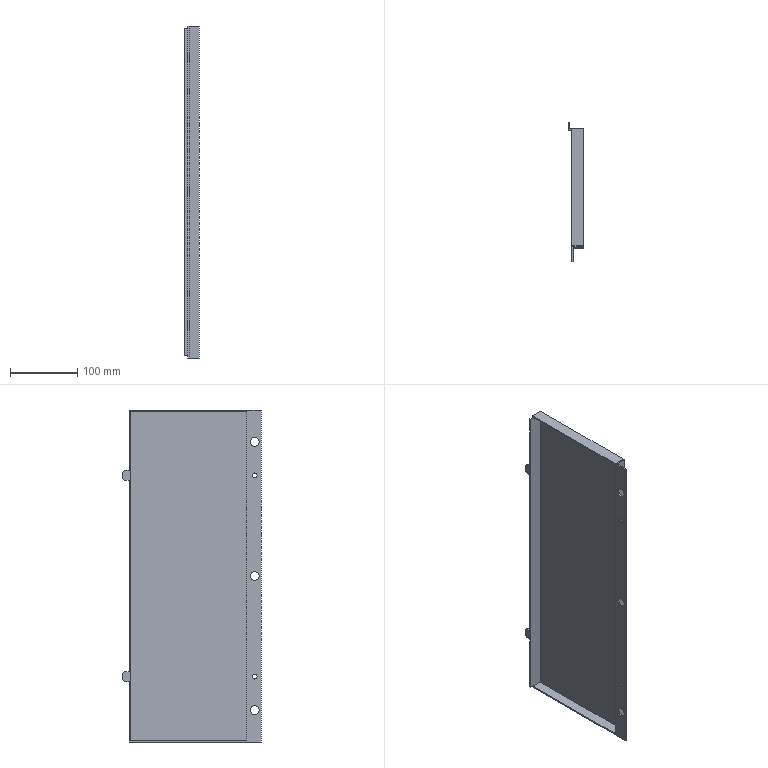Part | SolidWorks | features BaseBody 1 | 1 solid | 42 faces | box 22 x 207 x 495 mm | volume 239502 mm3 | plane 32 | cylinder 10 | commonest cylinder face diameters 13.1 x6 7.2 x4
STEP:
#1=CARTESIAN_POINT('',(194.446,-4330.973,706.371));
#2=VERTEX_POINT('',#1);
#3=CARTESIAN_POINT('',(194.446,-4330.973,713.571));
#4=VERTEX_POINT('',#3);
#5=CARTESIAN_POINT('',(194.446,-4330.973,709.971));
#6=DIRECTION('',(-1.,0.,0.));
#7=DIRECTION('',(0.,0.,1.));
#8=AXIS2_PLACEMENT_3D('',#5,#6,#7);
#9=CIRCLE('',#8,3.6);
#10=EDGE_CURVE('',#2,#4,#9,.T.);
#11=ORIENTED_EDGE('',*,*,#10,.F.);
#12=CARTESIAN_POINT('',(192.446,-4330.973,706.371));
#13=VERTEX_POINT('',#12);
#14=CARTESIAN_POINT('',(201.592,-4330.973,706.371));
#15=DIRECTION('',(-1.,0.,0.));
#16=VECTOR('',#15,1000.);
#17=LINE('',#14,#16);
#18=EDGE_CURVE('',#2,#13,#17,.T.);
#19=ORIENTED_EDGE('',*,*,#18,.T.);
#20=CARTESIAN_POINT('',(192.446,-4330.973,713.571));
#21=VERTEX_POINT('',#20);
#22=CARTESIAN_POINT('',(192.446,-4330.973,709.971));
#23=DIRECTION('',(1.,0.,0.));
#24=DIRECTION('',(0.,0.,1.));
#25=AXIS2_PLACEMENT_3D('',#22,#23,#24);
#26=CIRCLE('',#25,3.6);
#27=EDGE_CURVE('',#21,#13,#26,.T.);
#28=ORIENTED_EDGE('',*,*,#27,.F.);
#29=CARTESIAN_POINT('',(201.592,-4330.973,713.571));
#30=DIRECTION('',(-1.,0.,0.));
#31=VECTOR('',#30,1000.);
#32=LINE('',#29,#31);
#33=EDGE_CURVE('',#4,#21,#32,.T.);
#34=ORIENTED_EDGE('',*,*,#33,.F.);
#35=EDGE_LOOP('',(#11,#19,#28,#34));
#36=FACE_OUTER_BOUND('',#35,.T.);
#37=CARTESIAN_POINT('',(201.592,-4330.973,709.971));
#38=DIRECTION('',(-1.,0.,0.));
#39=DIRECTION('',(0.,0.,1.));
#40=AXIS2_PLACEMENT_3D('',#37,#38,#39);
#41=CYLINDRICAL_SURFACE('',#40,3.6);
#42=ADVANCED_FACE('',(#36),#41,.F.);
#43=CARTESIAN_POINT('',(194.446,-4330.973,406.371));
#44=VERTEX_POINT('',#43);
#45=CARTESIAN_POINT('',(194.446,-4330.973,413.571));
#46=VERTEX_POINT('',#45);
#47=CARTESIAN_POINT('',(194.446,-4330.973,409.971));
#48=DIRECTION('',(-1.,0.,0.));
#49=DIRECTION('',(0.,0.,1.));
#50=AXIS2_PLACEMENT_3D('',#47,#48,#49);
#51=CIRCLE('',#50,3.6);
#52=EDGE_CURVE('',#44,#46,#51,.T.);
#53=ORIENTED_EDGE('',*,*,#52,.F.);
#54=CARTESIAN_POINT('',(192.446,-4330.973,406.371));
#55=VERTEX_POINT('',#54);
#56=CARTESIAN_POINT('',(201.592,-4330.973,406.371));
#57=DIRECTION('',(-1.,0.,0.));
#58=VECTOR('',#57,1000.);
#59=LINE('',#56,#58);
#60=EDGE_CURVE('',#44,#55,#59,.T.);
#61=ORIENTED_EDGE('',*,*,#60,.T.);
#62=CARTESIAN_POINT('',(192.446,-4330.973,413.571));
#63=VERTEX_POINT('',#62);
#64=CARTESIAN_POINT('',(192.446,-4330.973,409.971));
#65=DIRECTION('',(1.,0.,0.));
#66=DIRECTION('',(0.,0.,1.));
#67=AXIS2_PLACEMENT_3D('',#64,#65,#66);
#68=CIRCLE('',#67,3.6);
#69=EDGE_CURVE('',#63,#55,#68,.T.);
#70=ORIENTED_EDGE('',*,*,#69,.F.);
#71=CARTESIAN_POINT('',(201.592,-4330.973,413.571));
#72=DIRECTION('',(-1.,0.,0.));
#73=VECTOR('',#72,1000.);
#74=LINE('',#71,#73);
#75=EDGE_CURVE('',#46,#63,#74,.T.);
#76=ORIENTED_EDGE('',*,*,#75,.F.);
#77=EDGE_LOOP('',(#53,#61,#70,#76));
#78=FACE_OUTER_BOUND('',#77,.T.);
#79=CARTESIAN_POINT('',(201.592,-4330.973,409.971));
#80=DIRECTION('',(-1.,0.,0.));
#81=DIRECTION('',(0.,0.,1.));
#82=AXIS2_PLACEMENT_3D('',#79,#80,#81);
#83=CYLINDRICAL_SURFACE('',#82,3.6);
#84=ADVANCED_FACE('',(#78),#83,.F.);
#85=CARTESIAN_POINT('',(194.446,-4330.973,353.421));
#86=VERTEX_POINT('',#85);
#87=CARTESIAN_POINT('',(194.446,-4330.973,366.521));
#88=VERTEX_POINT('',#87);
#89=CARTESIAN_POINT('',(194.446,-4330.973,359.971));
#90=DIRECTION('',(-1.,0.,0.));
#91=DIRECTION('',(0.,0.,1.));
#92=AXIS2_PLACEMENT_3D('',#89,#90,#91);
#93=CIRCLE('',#92,6.55);
#94=EDGE_CURVE('',#86,#88,#93,.T.);
#95=ORIENTED_EDGE('',*,*,#94,.F.);
#96=CARTESIAN_POINT('',(192.446,-4330.973,353.421));
#97=VERTEX_POINT('',#96);
#98=CARTESIAN_POINT('',(212.499,-4330.973,353.421));
#99=DIRECTION('',(-1.,0.,0.));
#100=VECTOR('',#99,1000.);
#101=LINE('',#98,#100);
#102=EDGE_CURVE('',#86,#97,#101,.T.);
#103=ORIENTED_EDGE('',*,*,#102,.T.);
#104=CARTESIAN_POINT('',(192.446,-4330.973,366.521));
#105=VERTEX_POINT('',#104);
#106=CARTESIAN_POINT('',(192.446,-4330.973,359.971));
#107=DIRECTION('',(1.,0.,0.));
#108=DIRECTION('',(0.,0.,1.));
#109=AXIS2_PLACEMENT_3D('',#106,#107,#108);
#110=CIRCLE('',#109,6.55);
#111=EDGE_CURVE('',#105,#97,#110,.T.);
#112=ORIENTED_EDGE('',*,*,#111,.F.);
#113=CARTESIAN_POINT('',(212.499,-4330.973,366.521));
#114=DIRECTION('',(-1.,0.,0.));
#115=VECTOR('',#114,1000.);
#116=LINE('',#113,#115);
#117=EDGE_CURVE('',#88,#105,#116,.T.);
#118=ORIENTED_EDGE('',*,*,#117,.F.);
#119=EDGE_LOOP('',(#95,#103,#112,#118));
#120=FACE_OUTER_BOUND('',#119,.T.);
#121=CARTESIAN_POINT('',(212.499,-4330.973,359.971));
#122=DIRECTION('',(-1.,0.,0.));
#123=DIRECTION('',(0.,0.,1.));
#124=AXIS2_PLACEMENT_3D('',#121,#122,#123);
#125=CYLINDRICAL_SURFACE('',#124,6.55);
#126=ADVANCED_FACE('',(#120),#125,.F.);
#127=CARTESIAN_POINT('',(194.446,-4330.973,753.421));
#128=VERTEX_POINT('',#127);
#129=CARTESIAN_POINT('',(194.446,-4330.973,766.521));
#130=VERTEX_POINT('',#129);
#131=CARTESIAN_POINT('',(194.446,-4330.973,759.971));
#132=DIRECTION('',(-1.,0.,0.));
#133=DIRECTION('',(0.,0.,1.));
#134=AXIS2_PLACEMENT_3D('',#131,#132,#133);
#135=CIRCLE('',#134,6.55);
#136=EDGE_CURVE('',#128,#130,#135,.T.);
#137=ORIENTED_EDGE('',*,*,#136,.F.);
#138=CARTESIAN_POINT('',(192.446,-4330.973,753.421));
#139=VERTEX_POINT('',#138);
#140=CARTESIAN_POINT('',(210.499,-4330.973,753.421));
#141=DIRECTION('',(-1.,0.,0.));
#142=VECTOR('',#141,1000.);
#143=LINE('',#140,#142);
#144=EDGE_CURVE('',#128,#139,#143,.T.);
#145=ORIENTED_EDGE('',*,*,#144,.T.);
#146=CARTESIAN_POINT('',(192.446,-4330.973,766.521));
#147=VERTEX_POINT('',#146);
#148=CARTESIAN_POINT('',(192.446,-4330.973,759.971));
#149=DIRECTION('',(1.,0.,0.));
#150=DIRECTION('',(0.,0.,1.));
#151=AXIS2_PLACEMENT_3D('',#148,#149,#150);
#152=CIRCLE('',#151,6.55);
#153=EDGE_CURVE('',#147,#139,#152,.T.);
#154=ORIENTED_EDGE('',*,*,#153,.F.);
#155=CARTESIAN_POINT('',(210.499,-4330.973,766.521));
#156=DIRECTION('',(-1.,0.,0.));
#157=VECTOR('',#156,1000.);
#158=LINE('',#155,#157);
#159=EDGE_CURVE('',#130,#147,#158,.T.);
#160=ORIENTED_EDGE('',*,*,#159,.F.);
#161=EDGE_LOOP('',(#137,#145,#154,#160));
#162=FACE_OUTER_BOUND('',#161,.T.);
#163=CARTESIAN_POINT('',(210.499,-4330.973,759.971));
#164=DIRECTION('',(-1.,0.,0.));
#165=DIRECTION('',(0.,0.,1.));
#166=AXIS2_PLACEMENT_3D('',#163,#164,#165);
#167=CYLINDRICAL_SURFACE('',#166,6.55);
#168=ADVANCED_FACE('',(#162),#167,.F.);
#169=CARTESIAN_POINT('',(194.446,-4330.973,553.421));
#170=VERTEX_POINT('',#169);
#171=CARTESIAN_POINT('',(194.446,-4330.973,566.521));
#172=VERTEX_POINT('',#171);
#173=CARTESIAN_POINT('',(194.446,-4330.973,559.971));
#174=DIRECTION('',(-1.,0.,0.));
#175=DIRECTION('',(0.,0.,1.));
#176=AXIS2_PLACEMENT_3D('',#173,#174,#175);
#177=CIRCLE('',#176,6.55);
#178=EDGE_CURVE('',#170,#172,#177,.T.);
#179=ORIENTED_EDGE('',*,*,#178,.F.);
#180=CARTESIAN_POINT('',(192.446,-4330.973,553.421));
#181=VERTEX_POINT('',#180);
#182=CARTESIAN_POINT('',(212.499,-4330.973,553.421));
#183=DIRECTION('',(-1.,0.,0.));
#184=VECTOR('',#183,1000.);
#185=LINE('',#182,#184);
#186=EDGE_CURVE('',#170,#181,#185,.T.);
#187=ORIENTED_EDGE('',*,*,#186,.T.);
#188=CARTESIAN_POINT('',(192.446,-4330.973,566.521));
#189=VERTEX_POINT('',#188);
#190=CARTESIAN_POINT('',(192.446,-4330.973,559.971));
#191=DIRECTION('',(1.,0.,0.));
#192=DIRECTION('',(0.,0.,1.));
#193=AXIS2_PLACEMENT_3D('',#190,#191,#192);
#194=CIRCLE('',#193,6.55);
#195=EDGE_CURVE('',#189,#181,#194,.T.);
#196=ORIENTED_EDGE('',*,*,#195,.F.);
#197=CARTESIAN_POINT('',(212.499,-4330.973,566.521));
#198=DIRECTION('',(-1.,0.,0.));
#199=VECTOR('',#198,1000.);
#200=LINE('',#197,#199);
#201=EDGE_CURVE('',#172,#189,#200,.T.);
#202=ORIENTED_EDGE('',*,*,#201,.F.);
#203=EDGE_LOOP('',(#179,#187,#196,#202));
#204=FACE_OUTER_BOUND('',#203,.T.);
#205=CARTESIAN_POINT('',(212.499,-4330.973,559.971));
#206=DIRECTION('',(-1.,0.,0.));
#207=DIRECTION('',(0.,0.,1.));
#208=AXIS2_PLACEMENT_3D('',#205,#206,#207);
#209=CYLINDRICAL_SURFACE('',#208,6.55);
#210=ADVANCED_FACE('',(#204),#209,.F.);
#211=CARTESIAN_POINT('',(209.446,-4320.973,312.471));
#212=VERTEX_POINT('',#211);
#213=CARTESIAN_POINT('',(209.446,-4143.973,312.471));
#214=VERTEX_POINT('',#213);
#215=CARTESIAN_POINT('',(209.446,-4143.973,312.471));
#216=DIRECTION('',(0.,1.,0.));
#217=VECTOR('',#216,1000.);
#218=LINE('',#215,#217);
#219=EDGE_CURVE('',#212,#214,#218,.T.);
#220=ORIENTED_EDGE('',*,*,#219,.T.);
#221=CARTESIAN_POINT('',(209.446,-4143.973,807.471));
#222=VERTEX_POINT('',#221);
#223=CARTESIAN_POINT('',(209.446,-4143.973,207.471));
#224=DIRECTION('',(0.,0.,1.));
#225=VECTOR('',#224,1000.);
#226=LINE('',#223,#225);
#227=EDGE_CURVE('',#214,#222,#226,.T.);
#228=ORIENTED_EDGE('',*,*,#227,.T.);
#229=CARTESIAN_POINT('',(209.446,-4320.973,807.471));
#230=VERTEX_POINT('',#229);
#231=CARTESIAN_POINT('',(209.446,-4143.973,807.471));
#232=DIRECTION('',(0.,-1.,0.));
#233=VECTOR('',#232,1000.);
#234=LINE('',#231,#233);
#235=EDGE_CURVE('',#222,#230,#234,.T.);
#236=ORIENTED_EDGE('',*,*,#235,.T.);
#237=CARTESIAN_POINT('',(209.446,-4320.973,207.471));
#238=DIRECTION('',(0.,0.,-1.));
#239=VECTOR('',#238,1000.);
#240=LINE('',#237,#239);
#241=EDGE_CURVE('',#230,#212,#240,.T.);
#242=ORIENTED_EDGE('',*,*,#241,.T.);
#243=EDGE_LOOP('',(#220,#228,#236,#242));
#244=FACE_OUTER_BOUND('',#243,.T.);
#245=CARTESIAN_POINT('',(209.446,-4143.973,207.471));
#246=DIRECTION('',(1.,0.,0.));
#247=DIRECTION('',(0.,0.,-1.));
#248=AXIS2_PLACEMENT_3D('',#245,#246,#247);
#249=PLANE('',#248);
#250=ADVANCED_FACE('',(#244),#249,.T.);
#251=CARTESIAN_POINT('',(187.446,-4143.973,402.471));
#252=VERTEX_POINT('',#251);
#253=CARTESIAN_POINT('',(189.446,-4143.973,402.471));
#254=VERTEX_POINT('',#253);
#255=CARTESIAN_POINT('',(207.446,-4143.973,402.471));
#256=DIRECTION('',(1.,0.,0.));
#257=VECTOR('',#256,1000.);
#258=LINE('',#255,#257);
#259=EDGE_CURVE('',#252,#254,#258,.T.);
#260=ORIENTED_EDGE('',*,*,#259,.T.);
#261=CARTESIAN_POINT('',(189.446,-4143.973,417.471));
#262=VERTEX_POINT('',#261);
#263=CARTESIAN_POINT('',(189.446,-4143.973,910.471));
#264=DIRECTION('',(0.,0.,1.));
#265=VECTOR('',#264,1000.);
#266=LINE('',#263,#265);
#267=EDGE_CURVE('',#254,#262,#266,.T.);
#268=ORIENTED_EDGE('',*,*,#267,.T.);
#269=CARTESIAN_POINT('',(187.446,-4143.973,417.471));
#270=VERTEX_POINT('',#269);
#271=CARTESIAN_POINT('',(207.446,-4143.973,417.471));
#272=DIRECTION('',(-1.,0.,0.));
#273=VECTOR('',#272,1000.);
#274=LINE('',#271,#273);
#275=EDGE_CURVE('',#262,#270,#274,.T.);
#276=ORIENTED_EDGE('',*,*,#275,.T.);
#277=CARTESIAN_POINT('',(187.446,-4143.973,702.471));
#278=VERTEX_POINT('',#277);
#279=CARTESIAN_POINT('',(187.446,-4143.973,910.471));
#280=DIRECTION('',(0.,0.,1.));
#281=VECTOR('',#280,1000.);
#282=LINE('',#279,#281);
#283=EDGE_CURVE('',#270,#278,#282,.T.);
#284=ORIENTED_EDGE('',*,*,#283,.T.);
#285=CARTESIAN_POINT('',(189.446,-4143.973,702.471));
#286=VERTEX_POINT('',#285);
#287=CARTESIAN_POINT('',(207.446,-4143.973,702.471));
#288=DIRECTION('',(1.,0.,0.));
#289=VECTOR('',#288,1000.);
#290=LINE('',#287,#289);
#291=EDGE_CURVE('',#278,#286,#290,.T.);
#292=ORIENTED_EDGE('',*,*,#291,.T.);
#293=CARTESIAN_POINT('',(189.446,-4143.973,717.471));
#294=VERTEX_POINT('',#293);
#295=CARTESIAN_POINT('',(189.446,-4143.973,910.471));
#296=DIRECTION('',(0.,0.,1.));
#297=VECTOR('',#296,1000.);
#298=LINE('',#295,#297);
#299=EDGE_CURVE('',#286,#294,#298,.T.);
#300=ORIENTED_EDGE('',*,*,#299,.T.);
#301=CARTESIAN_POINT('',(187.446,-4143.973,717.471));
#302=VERTEX_POINT('',#301);
#303=CARTESIAN_POINT('',(207.446,-4143.973,717.471));
#304=DIRECTION('',(-1.,0.,0.));
#305=VECTOR('',#304,1000.);
#306=LINE('',#303,#305);
#307=EDGE_CURVE('',#294,#302,#306,.T.);
#308=ORIENTED_EDGE('',*,*,#307,.T.);
#309=CARTESIAN_POINT('',(187.446,-4143.973,804.471));
#310=VERTEX_POINT('',#309);
#311=CARTESIAN_POINT('',(187.446,-4143.973,910.471));
#312=DIRECTION('',(0.,0.,1.));
#313=VECTOR('',#312,1000.);
#314=LINE('',#311,#313);
#315=EDGE_CURVE('',#302,#310,#314,.T.);
#316=ORIENTED_EDGE('',*,*,#315,.T.);
#317=CARTESIAN_POINT('',(207.446,-4143.973,804.471));
#318=VERTEX_POINT('',#317);
#319=CARTESIAN_POINT('',(207.446,-4143.973,804.471));
#320=DIRECTION('',(1.,0.,0.));
#321=VECTOR('',#320,1000.);
#322=LINE('',#319,#321);
#323=EDGE_CURVE('',#310,#318,#322,.T.);
#324=ORIENTED_EDGE('',*,*,#323,.T.);
#325=CARTESIAN_POINT('',(207.446,-4143.973,805.471));
#326=VERTEX_POINT('',#325);
#327=CARTESIAN_POINT('',(207.446,-4143.973,207.471));
#328=DIRECTION('',(0.,0.,-1.));
#329=VECTOR('',#328,1000.);
#330=LINE('',#327,#329);
#331=EDGE_CURVE('',#326,#318,#330,.T.);
#332=ORIENTED_EDGE('',*,*,#331,.F.);
#333=CARTESIAN_POINT('',(192.446,-4143.973,805.471));
#334=VERTEX_POINT('',#333);
#335=CARTESIAN_POINT('',(207.446,-4143.973,805.471));
#336=DIRECTION('',(-1.,0.,0.));
#337=VECTOR('',#336,1000.);
#338=LINE('',#335,#337);
#339=EDGE_CURVE('',#326,#334,#338,.T.);
#340=ORIENTED_EDGE('',*,*,#339,.T.);
#341=CARTESIAN_POINT('',(192.446,-4143.973,807.471));
#342=VERTEX_POINT('',#341);
#343=CARTESIAN_POINT('',(192.446,-4143.973,910.471));
#344=DIRECTION('',(0.,0.,1.));
#345=VECTOR('',#344,1000.);
#346=LINE('',#343,#345);
#347=EDGE_CURVE('',#334,#342,#346,.T.);
#348=ORIENTED_EDGE('',*,*,#347,.T.);
#349=CARTESIAN_POINT('',(207.446,-4143.973,807.471));
#350=DIRECTION('',(1.,0.,0.));
#351=VECTOR('',#350,1000.);
#352=LINE('',#349,#351);
#353=EDGE_CURVE('',#342,#222,#352,.T.);
#354=ORIENTED_EDGE('',*,*,#353,.T.);
#355=ORIENTED_EDGE('',*,*,#227,.F.);
#356=CARTESIAN_POINT('',(192.446,-4143.973,312.471));
#357=VERTEX_POINT('',#356);
#358=CARTESIAN_POINT('',(207.446,-4143.973,312.471));
#359=DIRECTION('',(-1.,0.,0.));
#360=VECTOR('',#359,1000.);
#361=LINE('',#358,#360);
#362=EDGE_CURVE('',#214,#357,#361,.T.);
#363=ORIENTED_EDGE('',*,*,#362,.T.);
#364=CARTESIAN_POINT('',(192.446,-4143.973,314.471));
#365=VERTEX_POINT('',#364);
#366=CARTESIAN_POINT('',(192.446,-4143.973,910.471));
#367=DIRECTION('',(0.,0.,1.));
#368=VECTOR('',#367,1000.);
#369=LINE('',#366,#368);
#370=EDGE_CURVE('',#357,#365,#369,.T.);
#371=ORIENTED_EDGE('',*,*,#370,.T.);
#372=CARTESIAN_POINT('',(207.446,-4143.973,314.471));
#373=VERTEX_POINT('',#372);
#374=CARTESIAN_POINT('',(207.446,-4143.973,314.471));
#375=DIRECTION('',(1.,0.,0.));
#376=VECTOR('',#375,1000.);
#377=LINE('',#374,#376);
#378=EDGE_CURVE('',#365,#373,#377,.T.);
#379=ORIENTED_EDGE('',*,*,#378,.T.);
#380=CARTESIAN_POINT('',(207.446,-4143.973,315.471));
#381=VERTEX_POINT('',#380);
#382=CARTESIAN_POINT('',(207.446,-4143.973,207.471));
#383=DIRECTION('',(0.,0.,-1.));
#384=VECTOR('',#383,1000.);
#385=LINE('',#382,#384);
#386=EDGE_CURVE('',#381,#373,#385,.T.);
#387=ORIENTED_EDGE('',*,*,#386,.F.);
#388=CARTESIAN_POINT('',(187.446,-4143.973,315.471));
#389=VERTEX_POINT('',#388);
#390=CARTESIAN_POINT('',(207.446,-4143.973,315.471));
#391=DIRECTION('',(-1.,0.,0.));
#392=VECTOR('',#391,1000.);
#393=LINE('',#390,#392);
#394=EDGE_CURVE('',#381,#389,#393,.T.);
#395=ORIENTED_EDGE('',*,*,#394,.T.);
#396=CARTESIAN_POINT('',(187.446,-4143.973,910.471));
#397=DIRECTION('',(0.,0.,1.));
#398=VECTOR('',#397,1000.);
#399=LINE('',#396,#398);
#400=EDGE_CURVE('',#389,#252,#399,.T.);
#401=ORIENTED_EDGE('',*,*,#400,.T.);
#402=EDGE_LOOP('',(#260,#268,#276,#284,#292,#300,#308,#316,#324,#332,#340,#348,#354,#355,#363,#371,#379,#387,#395,#401));
#403=FACE_OUTER_BOUND('',#402,.T.);
#404=CARTESIAN_POINT('',(207.446,-4143.973,910.471));
#405=DIRECTION('',(0.,1.,0.));
#406=DIRECTION('',(0.,0.,1.));
#407=AXIS2_PLACEMENT_3D('',#404,#405,#406);
#408=PLANE('',#407);
#409=ADVANCED_FACE('',(#403),#408,.T.);
#410=CARTESIAN_POINT('',(207.446,-4318.473,312.471));
#411=VERTEX_POINT('',#410);
#412=CARTESIAN_POINT('',(207.446,-4318.973,312.471));
#413=VERTEX_POINT('',#412);
#414=CARTESIAN_POINT('',(207.446,-4318.973,312.471));
#415=DIRECTION('',(0.,-1.,0.));
#416=VECTOR('',#415,1000.);
#417=LINE('',#414,#416);
#418=EDGE_CURVE('',#411,#413,#417,.T.);
#419=ORIENTED_EDGE('',*,*,#418,.F.);
#420=CARTESIAN_POINT('',(192.446,-4318.473,312.471));
#421=VERTEX_POINT('',#420);
#422=CARTESIAN_POINT('',(207.446,-4318.473,312.471));
#423=DIRECTION('',(-1.,0.,0.));
#424=VECTOR('',#423,1000.);
#425=LINE('',#422,#424);
#426=EDGE_CURVE('',#411,#421,#425,.T.);
#427=ORIENTED_EDGE('',*,*,#426,.T.);
#428=CARTESIAN_POINT('',(192.446,-4143.973,312.471));
#429=DIRECTION('',(0.,1.,0.));
#430=VECTOR('',#429,1000.);
#431=LINE('',#428,#430);
#432=EDGE_CURVE('',#421,#357,#431,.T.);
#433=ORIENTED_EDGE('',*,*,#432,.T.);
#434=ORIENTED_EDGE('',*,*,#362,.F.);
#435=ORIENTED_EDGE('',*,*,#219,.F.);
#436=CARTESIAN_POINT('',(194.446,-4320.973,312.471));
#437=VERTEX_POINT('',#436);
#438=CARTESIAN_POINT('',(207.446,-4320.973,312.471));
#439=DIRECTION('',(-1.,0.,0.));
#440=VECTOR('',#439,1000.);
#441=LINE('',#438,#440);
#442=EDGE_CURVE('',#212,#437,#441,.T.);
#443=ORIENTED_EDGE('',*,*,#442,.T.);
#444=CARTESIAN_POINT('',(194.446,-4340.973,312.471));
#445=VERTEX_POINT('',#444);
#446=CARTESIAN_POINT('',(194.446,-4143.973,312.471));
#447=DIRECTION('',(0.,-1.,0.));
#448=VECTOR('',#447,1000.);
#449=LINE('',#446,#448);
#450=EDGE_CURVE('',#437,#445,#449,.T.);
#451=ORIENTED_EDGE('',*,*,#450,.T.);
#452=CARTESIAN_POINT('',(192.446,-4340.973,312.471));
#453=VERTEX_POINT('',#452);
#454=CARTESIAN_POINT('',(207.446,-4340.973,312.471));
#455=DIRECTION('',(-1.,0.,0.));
#456=VECTOR('',#455,1000.);
#457=LINE('',#454,#456);
#458=EDGE_CURVE('',#445,#453,#457,.T.);
#459=ORIENTED_EDGE('',*,*,#458,.T.);
#460=CARTESIAN_POINT('',(192.446,-4318.973,312.471));
#461=VERTEX_POINT('',#460);
#462=CARTESIAN_POINT('',(192.446,-4143.973,312.471));
#463=DIRECTION('',(0.,1.,0.));
#464=VECTOR('',#463,1000.);
#465=LINE('',#462,#464);
#466=EDGE_CURVE('',#453,#461,#465,.T.);
#467=ORIENTED_EDGE('',*,*,#466,.T.);
#468=CARTESIAN_POINT('',(207.446,-4318.973,312.471));
#469=DIRECTION('',(1.,0.,0.));
#470=VECTOR('',#469,1000.);
#471=LINE('',#468,#470);
#472=EDGE_CURVE('',#461,#413,#471,.T.);
#473=ORIENTED_EDGE('',*,*,#472,.T.);
#474=EDGE_LOOP('',(#419,#427,#433,#434,#435,#443,#451,#459,#467,#473));
#475=FACE_OUTER_BOUND('',#474,.T.);
#476=CARTESIAN_POINT('',(207.446,-4143.973,312.471));
#477=DIRECTION('',(0.,0.,-1.));
#478=DIRECTION('',(-1.,0.,0.));
#479=AXIS2_PLACEMENT_3D('',#476,#477,#478);
#480=PLANE('',#479);
#481=ADVANCED_FACE('',(#475),#480,.T.);
#482=ORIENTED_EDGE('',*,*,#442,.F.);
#483=ORIENTED_EDGE('',*,*,#241,.F.);
#484=CARTESIAN_POINT('',(194.446,-4320.973,807.471));
#485=VERTEX_POINT('',#484);
#486=CARTESIAN_POINT('',(209.446,-4320.973,807.471));
#487=DIRECTION('',(-1.,0.,0.));
#488=VECTOR('',#487,1000.);
#489=LINE('',#486,#488);
#490=EDGE_CURVE('',#230,#485,#489,.T.);
#491=ORIENTED_EDGE('',*,*,#490,.T.);
#492=CARTESIAN_POINT('',(194.446,-4320.973,207.471));
#493=DIRECTION('',(0.,0.,-1.));
#494=VECTOR('',#493,1000.);
#495=LINE('',#492,#494);
#496=EDGE_CURVE('',#485,#437,#495,.T.);
#497=ORIENTED_EDGE('',*,*,#496,.T.);
#498=EDGE_LOOP('',(#482,#483,#491,#497));
#499=FACE_OUTER_BOUND('',#498,.T.);
#500=CARTESIAN_POINT('',(209.446,-4320.973,207.471));
#501=DIRECTION('',(0.,-1.,0.));
#502=DIRECTION('',(0.,0.,-1.));
#503=AXIS2_PLACEMENT_3D('',#500,#501,#502);
#504=PLANE('',#503);
#505=ADVANCED_FACE('',(#499),#504,.T.);
#506=ORIENTED_EDGE('',*,*,#235,.F.);
#507=ORIENTED_EDGE('',*,*,#353,.F.);
#508=CARTESIAN_POINT('',(192.446,-4318.473,807.471));
#509=VERTEX_POINT('',#508);
#510=CARTESIAN_POINT('',(192.446,-4143.973,807.471));
#511=DIRECTION('',(0.,-1.,0.));
#512=VECTOR('',#511,1000.);
#513=LINE('',#510,#512);
#514=EDGE_CURVE('',#342,#509,#513,.T.);
#515=ORIENTED_EDGE('',*,*,#514,.T.);
#516=CARTESIAN_POINT('',(207.446,-4318.473,807.471));
#517=VERTEX_POINT('',#516);
#518=CARTESIAN_POINT('',(207.446,-4318.473,807.471));
#519=DIRECTION('',(1.,0.,0.));
#520=VECTOR('',#519,1000.);
#521=LINE('',#518,#520);
#522=EDGE_CURVE('',#509,#517,#521,.T.);
#523=ORIENTED_EDGE('',*,*,#522,.T.);
#524=CARTESIAN_POINT('',(207.446,-4318.973,807.471));
#525=VERTEX_POINT('',#524);
#526=CARTESIAN_POINT('',(207.446,-4318.973,807.471));
#527=DIRECTION('',(0.,1.,0.));
#528=VECTOR('',#527,1000.);
#529=LINE('',#526,#528);
#530=EDGE_CURVE('',#525,#517,#529,.T.);
#531=ORIENTED_EDGE('',*,*,#530,.F.);
#532=CARTESIAN_POINT('',(192.446,-4318.973,807.471));
#533=VERTEX_POINT('',#532);
#534=CARTESIAN_POINT('',(207.446,-4318.973,807.471));
#535=DIRECTION('',(-1.,0.,0.));
#536=VECTOR('',#535,1000.);
#537=LINE('',#534,#536);
#538=EDGE_CURVE('',#525,#533,#537,.T.);
#539=ORIENTED_EDGE('',*,*,#538,.T.);
#540=CARTESIAN_POINT('',(192.446,-4340.973,807.471));
#541=VERTEX_POINT('',#540);
#542=CARTESIAN_POINT('',(192.446,-4143.973,807.471));
#543=DIRECTION('',(0.,-1.,0.));
#544=VECTOR('',#543,1000.);
#545=LINE('',#542,#544);
#546=EDGE_CURVE('',#533,#541,#545,.T.);
#547=ORIENTED_EDGE('',*,*,#546,.T.);
#548=CARTESIAN_POINT('',(194.446,-4340.973,807.471));
#549=VERTEX_POINT('',#548);
#550=CARTESIAN_POINT('',(207.446,-4340.973,807.471));
#551=DIRECTION('',(1.,0.,0.));
#552=VECTOR('',#551,1000.);
#553=LINE('',#550,#552);
#554=EDGE_CURVE('',#541,#549,#553,.T.);
#555=ORIENTED_EDGE('',*,*,#554,.T.);
#556=CARTESIAN_POINT('',(194.446,-4143.973,807.471));
#557=DIRECTION('',(0.,1.,0.));
#558=VECTOR('',#557,1000.);
#559=LINE('',#556,#558);
#560=EDGE_CURVE('',#549,#485,#559,.T.);
#561=ORIENTED_EDGE('',*,*,#560,.T.);
#562=ORIENTED_EDGE('',*,*,#490,.F.);
#563=EDGE_LOOP('',(#506,#507,#515,#523,#531,#539,#547,#555,#561,#562));
#564=FACE_OUTER_BOUND('',#563,.T.);
#565=CARTESIAN_POINT('',(207.446,-4143.973,807.471));
#566=DIRECTION('',(0.,0.,1.));
#567=DIRECTION('',(1.,0.,0.));
#568=AXIS2_PLACEMENT_3D('',#565,#566,#567);
#569=PLANE('',#568);
#570=ADVANCED_FACE('',(#564),#569,.T.);
#571=CARTESIAN_POINT('',(189.446,-4133.973,414.471));
#572=VERTEX_POINT('',#571);
#573=CARTESIAN_POINT('',(189.446,-4136.973,417.471));
#574=VERTEX_POINT('',#573);
#575=CARTESIAN_POINT('',(189.446,-4133.973,414.471));
#576=DIRECTION('',(0.,-0.7071,0.7071));
#577=VECTOR('',#576,1000.);
#578=LINE('',#575,#577);
#579=EDGE_CURVE('',#572,#574,#578,.T.);
#580=ORIENTED_EDGE('',*,*,#579,.T.);
#581=CARTESIAN_POINT('',(189.446,-4140.465,417.471));
#582=DIRECTION('',(0.,-1.,0.));
#583=VECTOR('',#582,1000.);
#584=LINE('',#581,#583);
#585=EDGE_CURVE('',#574,#262,#584,.T.);
#586=ORIENTED_EDGE('',*,*,#585,.T.);
#587=ORIENTED_EDGE('',*,*,#267,.F.);
#588=CARTESIAN_POINT('',(189.446,-4136.973,402.471));
#589=VERTEX_POINT('',#588);
#590=CARTESIAN_POINT('',(189.446,-4140.465,402.471));
#591=DIRECTION('',(0.,1.,0.));
#592=VECTOR('',#591,1000.);
#593=LINE('',#590,#592);
#594=EDGE_CURVE('',#254,#589,#593,.T.);
#595=ORIENTED_EDGE('',*,*,#594,.T.);
#596=CARTESIAN_POINT('',(189.446,-4133.973,405.471));
#597=VERTEX_POINT('',#596);
#598=CARTESIAN_POINT('',(189.446,-4136.973,402.471));
#599=DIRECTION('',(0.,0.7071,0.7071));
#600=VECTOR('',#599,1000.);
#601=LINE('',#598,#600);
#602=EDGE_CURVE('',#589,#597,#601,.T.);
#603=ORIENTED_EDGE('',*,*,#602,.T.);
#604=CARTESIAN_POINT('',(189.446,-4133.973,439.971));
#605=DIRECTION('',(0.,0.,1.));
#606=VECTOR('',#605,1000.);
#607=LINE('',#604,#606);
#608=EDGE_CURVE('',#597,#572,#607,.T.);
#609=ORIENTED_EDGE('',*,*,#608,.T.);
#610=EDGE_LOOP('',(#580,#586,#587,#595,#603,#609));
#611=FACE_OUTER_BOUND('',#610,.T.);
#612=CARTESIAN_POINT('',(189.446,-4140.465,439.971));
#613=DIRECTION('',(1.,0.,0.));
#614=DIRECTION('',(0.,0.,-1.));
#615=AXIS2_PLACEMENT_3D('',#612,#613,#614);
#616=PLANE('',#615);
#617=ADVANCED_FACE('',(#611),#616,.T.);
#618=CARTESIAN_POINT('',(187.446,-4136.973,402.471));
#619=VERTEX_POINT('',#618);
#620=CARTESIAN_POINT('',(189.446,-4136.973,402.471));
#621=DIRECTION('',(1.,0.,0.));
#622=VECTOR('',#621,1000.);
#623=LINE('',#620,#622);
#624=EDGE_CURVE('',#619,#589,#623,.T.);
#625=ORIENTED_EDGE('',*,*,#624,.T.);
#626=ORIENTED_EDGE('',*,*,#594,.F.);
#627=ORIENTED_EDGE('',*,*,#259,.F.);
#628=CARTESIAN_POINT('',(187.446,-4145.973,402.471));
#629=DIRECTION('',(0.,1.,0.));
#630=VECTOR('',#629,1000.);
#631=LINE('',#628,#630);
#632=EDGE_CURVE('',#252,#619,#631,.T.);
#633=ORIENTED_EDGE('',*,*,#632,.T.);
#634=EDGE_LOOP('',(#625,#626,#627,#633));
#635=FACE_OUTER_BOUND('',#634,.T.);
#636=CARTESIAN_POINT('',(189.446,-4145.973,402.471));
#637=DIRECTION('',(0.,0.,-1.));
#638=DIRECTION('',(-1.,0.,0.));
#639=AXIS2_PLACEMENT_3D('',#636,#637,#638);
#640=PLANE('',#639);
#641=ADVANCED_FACE('',(#635),#640,.T.);
#642=CARTESIAN_POINT('',(187.446,-4133.973,414.471));
#643=VERTEX_POINT('',#642);
#644=CARTESIAN_POINT('',(187.446,-4136.973,417.471));
#645=VERTEX_POINT('',#644);
#646=CARTESIAN_POINT('',(187.446,-4133.973,414.471));
#647=DIRECTION('',(0.,-0.7071,0.7071));
#648=VECTOR('',#647,1000.);
#649=LINE('',#646,#648);
#650=EDGE_CURVE('',#643,#645,#649,.T.);
#651=ORIENTED_EDGE('',*,*,#650,.F.);
#652=CARTESIAN_POINT('',(187.446,-4133.973,405.471));
#653=VERTEX_POINT('',#652);
#654=CARTESIAN_POINT('',(187.446,-4133.973,484.971));
#655=DIRECTION('',(0.,0.,1.));
#656=VECTOR('',#655,1000.);
#657=LINE('',#654,#656);
#658=EDGE_CURVE('',#653,#643,#657,.T.);
#659=ORIENTED_EDGE('',*,*,#658,.F.);
#660=CARTESIAN_POINT('',(187.446,-4136.973,402.471));
#661=DIRECTION('',(0.,0.7071,0.7071));
#662=VECTOR('',#661,1000.);
#663=LINE('',#660,#662);
#664=EDGE_CURVE('',#619,#653,#663,.T.);
#665=ORIENTED_EDGE('',*,*,#664,.F.);
#666=ORIENTED_EDGE('',*,*,#632,.F.);
#667=ORIENTED_EDGE('',*,*,#400,.F.);
#668=CARTESIAN_POINT('',(187.446,-4145.973,315.471));
#669=VERTEX_POINT('',#668);
#670=CARTESIAN_POINT('',(187.446,-4140.465,315.471));
#671=DIRECTION('',(0.,1.,0.));
#672=VECTOR('',#671,1000.);
#673=LINE('',#670,#672);
#674=EDGE_CURVE('',#669,#389,#673,.T.);
#675=ORIENTED_EDGE('',*,*,#674,.F.);
#676=CARTESIAN_POINT('',(187.446,-4145.973,804.471));
#677=VERTEX_POINT('',#676);
#678=CARTESIAN_POINT('',(187.446,-4145.973,484.971));
#679=DIRECTION('',(0.,0.,-1.));
#680=VECTOR('',#679,1000.);
#681=LINE('',#678,#680);
#682=EDGE_CURVE('',#677,#669,#681,.T.);
#683=ORIENTED_EDGE('',*,*,#682,.F.);
#684=CARTESIAN_POINT('',(187.446,-4140.465,804.471));
#685=DIRECTION('',(0.,-1.,0.));
#686=VECTOR('',#685,1000.);
#687=LINE('',#684,#686);
#688=EDGE_CURVE('',#310,#677,#687,.T.);
#689=ORIENTED_EDGE('',*,*,#688,.F.);
#690=ORIENTED_EDGE('',*,*,#315,.F.);
#691=CARTESIAN_POINT('',(187.446,-4136.973,717.471));
#692=VERTEX_POINT('',#691);
#693=CARTESIAN_POINT('',(187.446,-4140.465,717.471));
#694=DIRECTION('',(0.,-1.,0.));
#695=VECTOR('',#694,1000.);
#696=LINE('',#693,#695);
#697=EDGE_CURVE('',#692,#302,#696,.T.);
#698=ORIENTED_EDGE('',*,*,#697,.F.);
#699=CARTESIAN_POINT('',(187.446,-4133.973,714.471));
#700=VERTEX_POINT('',#699);
#701=CARTESIAN_POINT('',(187.446,-4133.973,714.471));
#702=DIRECTION('',(0.,-0.7071,0.7071));
#703=VECTOR('',#702,1000.);
#704=LINE('',#701,#703);
#705=EDGE_CURVE('',#700,#692,#704,.T.);
#706=ORIENTED_EDGE('',*,*,#705,.F.);
#707=CARTESIAN_POINT('',(187.446,-4133.973,705.471));
#708=VERTEX_POINT('',#707);
#709=CARTESIAN_POINT('',(187.446,-4133.973,484.971));
#710=DIRECTION('',(0.,0.,1.));
#711=VECTOR('',#710,1000.);
#712=LINE('',#709,#711);
#713=EDGE_CURVE('',#708,#700,#712,.T.);
#714=ORIENTED_EDGE('',*,*,#713,.F.);
#715=CARTESIAN_POINT('',(187.446,-4136.973,702.471));
#716=VERTEX_POINT('',#715);
#717=CARTESIAN_POINT('',(187.446,-4136.973,702.471));
#718=DIRECTION('',(0.,0.7071,0.7071));
#719=VECTOR('',#718,1000.);
#720=LINE('',#717,#719);
#721=EDGE_CURVE('',#716,#708,#720,.T.);
#722=ORIENTED_EDGE('',*,*,#721,.F.);
#723=CARTESIAN_POINT('',(187.446,-4140.465,702.471));
#724=DIRECTION('',(0.,1.,0.));
#725=VECTOR('',#724,1000.);
#726=LINE('',#723,#725);
#727=EDGE_CURVE('',#278,#716,#726,.T.);
#728=ORIENTED_EDGE('',*,*,#727,.F.);
#729=ORIENTED_EDGE('',*,*,#283,.F.);
#730=CARTESIAN_POINT('',(187.446,-4140.465,417.471));
#731=DIRECTION('',(0.,-1.,0.));
#732=VECTOR('',#731,1000.);
#733=LINE('',#730,#732);
#734=EDGE_CURVE('',#645,#270,#733,.T.);
#735=ORIENTED_EDGE('',*,*,#734,.F.);
#736=EDGE_LOOP('',(#651,#659,#665,#666,#667,#675,#683,#689,#690,#698,#706,#714,#722,#728,#729,#735));
#737=FACE_OUTER_BOUND('',#736,.T.);
#738=CARTESIAN_POINT('',(187.446,-4140.465,484.971));
#739=DIRECTION('',(1.,0.,0.));
#740=DIRECTION('',(0.,0.,-1.));
#741=AXIS2_PLACEMENT_3D('',#738,#739,#740);
#742=PLANE('',#741);
#743=ADVANCED_FACE('',(#737),#742,.F.);
#744=CARTESIAN_POINT('',(207.446,-4145.973,315.471));
#745=VERTEX_POINT('',#744);
#746=CARTESIAN_POINT('',(207.446,-3995.973,315.471));
#747=DIRECTION('',(0.,1.,0.));
#748=VECTOR('',#747,1000.);
#749=LINE('',#746,#748);
#750=EDGE_CURVE('',#745,#381,#749,.T.);
#751=ORIENTED_EDGE('',*,*,#750,.F.);
#752=CARTESIAN_POINT('',(207.446,-4145.973,315.471));
#753=DIRECTION('',(1.,0.,0.));
#754=VECTOR('',#753,1000.);
#755=LINE('',#752,#754);
#756=EDGE_CURVE('',#669,#745,#755,.T.);
#757=ORIENTED_EDGE('',*,*,#756,.F.);
#758=ORIENTED_EDGE('',*,*,#674,.T.);
#759=ORIENTED_EDGE('',*,*,#394,.F.);
#760=EDGE_LOOP('',(#751,#757,#758,#759));
#761=FACE_OUTER_BOUND('',#760,.T.);
#762=CARTESIAN_POINT('',(207.446,-3995.973,315.471));
#763=DIRECTION('',(0.,0.,1.));
#764=DIRECTION('',(1.,0.,0.));
#765=AXIS2_PLACEMENT_3D('',#762,#763,#764);
#766=PLANE('',#765);
#767=ADVANCED_FACE('',(#761),#766,.F.);
#768=CARTESIAN_POINT('',(207.446,-4318.473,314.471));
#769=VERTEX_POINT('',#768);
#770=CARTESIAN_POINT('',(207.446,-4318.473,314.471));
#771=DIRECTION('',(0.,1.,0.));
#772=VECTOR('',#771,1000.);
#773=LINE('',#770,#772);
#774=EDGE_CURVE('',#769,#373,#773,.T.);
#775=ORIENTED_EDGE('',*,*,#774,.T.);
#776=ORIENTED_EDGE('',*,*,#378,.F.);
#777=CARTESIAN_POINT('',(192.446,-4318.473,314.471));
#778=VERTEX_POINT('',#777);
#779=CARTESIAN_POINT('',(192.446,-4318.473,314.471));
#780=DIRECTION('',(0.,-1.,0.));
#781=VECTOR('',#780,1000.);
#782=LINE('',#779,#781);
#783=EDGE_CURVE('',#365,#778,#782,.T.);
#784=ORIENTED_EDGE('',*,*,#783,.T.);
#785=CARTESIAN_POINT('',(207.446,-4318.473,314.471));
#786=DIRECTION('',(1.,0.,0.));
#787=VECTOR('',#786,1000.);
#788=LINE('',#785,#787);
#789=EDGE_CURVE('',#778,#769,#788,.T.);
#790=ORIENTED_EDGE('',*,*,#789,.T.);
#791=EDGE_LOOP('',(#775,#776,#784,#790));
#792=FACE_OUTER_BOUND('',#791,.T.);
#793=CARTESIAN_POINT('',(207.446,-4318.473,314.471));
#794=DIRECTION('',(0.,0.,1.));
#795=DIRECTION('',(1.,0.,0.));
#796=AXIS2_PLACEMENT_3D('',#793,#794,#795);
#797=PLANE('',#796);
#798=ADVANCED_FACE('',(#792),#797,.T.);
#799=ORIENTED_EDGE('',*,*,#432,.F.);
#800=CARTESIAN_POINT('',(192.446,-4318.473,208.471));
#801=DIRECTION('',(0.,0.,-1.));
#802=VECTOR('',#801,1000.);
#803=LINE('',#800,#802);
#804=EDGE_CURVE('',#778,#421,#803,.T.);
#805=ORIENTED_EDGE('',*,*,#804,.F.);
#806=ORIENTED_EDGE('',*,*,#783,.F.);
#807=ORIENTED_EDGE('',*,*,#370,.F.);
#808=EDGE_LOOP('',(#799,#805,#806,#807));
#809=FACE_OUTER_BOUND('',#808,.T.);
#810=CARTESIAN_POINT('',(192.446,-4231.223,208.471));
#811=DIRECTION('',(1.,0.,0.));
#812=DIRECTION('',(0.,0.,-1.));
#813=AXIS2_PLACEMENT_3D('',#810,#811,#812);
#814=PLANE('',#813);
#815=ADVANCED_FACE('',(#809),#814,.F.);
#816=CARTESIAN_POINT('',(192.446,-4318.473,805.471));
#817=VERTEX_POINT('',#816);
#818=CARTESIAN_POINT('',(192.446,-4231.223,805.471));
#819=DIRECTION('',(0.,1.,0.));
#820=VECTOR('',#819,1000.);
#821=LINE('',#818,#820);
#822=EDGE_CURVE('',#817,#334,#821,.T.);
#823=ORIENTED_EDGE('',*,*,#822,.F.);
#824=CARTESIAN_POINT('',(192.446,-4318.473,806.471));
#825=DIRECTION('',(0.,0.,-1.));
#826=VECTOR('',#825,1000.);
#827=LINE('',#824,#826);
#828=EDGE_CURVE('',#509,#817,#827,.T.);
#829=ORIENTED_EDGE('',*,*,#828,.F.);
#830=ORIENTED_EDGE('',*,*,#514,.F.);
#831=ORIENTED_EDGE('',*,*,#347,.F.);
#832=EDGE_LOOP('',(#823,#829,#830,#831));
#833=FACE_OUTER_BOUND('',#832,.T.);
#834=CARTESIAN_POINT('',(192.446,-4231.223,806.471));
#835=DIRECTION('',(1.,0.,0.));
#836=DIRECTION('',(0.,0.,-1.));
#837=AXIS2_PLACEMENT_3D('',#834,#835,#836);
#838=PLANE('',#837);
#839=ADVANCED_FACE('',(#833),#838,.F.);
#840=CARTESIAN_POINT('',(207.446,-4318.473,805.471));
#841=VERTEX_POINT('',#840);
#842=CARTESIAN_POINT('',(207.446,-4318.473,805.471));
#843=DIRECTION('',(0.,-1.,0.));
#844=VECTOR('',#843,1000.);
#845=LINE('',#842,#844);
#846=EDGE_CURVE('',#326,#841,#845,.T.);
#847=ORIENTED_EDGE('',*,*,#846,.T.);
#848=CARTESIAN_POINT('',(207.446,-4318.473,805.471));
#849=DIRECTION('',(-1.,0.,0.));
#850=VECTOR('',#849,1000.);
#851=LINE('',#848,#850);
#852=EDGE_CURVE('',#841,#817,#851,.T.);
#853=ORIENTED_EDGE('',*,*,#852,.T.);
#854=ORIENTED_EDGE('',*,*,#822,.T.);
#855=ORIENTED_EDGE('',*,*,#339,.F.);
#856=EDGE_LOOP('',(#847,#853,#854,#855));
#857=FACE_OUTER_BOUND('',#856,.T.);
#858=CARTESIAN_POINT('',(207.446,-4318.473,805.471));
#859=DIRECTION('',(0.,0.,-1.));
#860=DIRECTION('',(-1.,0.,0.));
#861=AXIS2_PLACEMENT_3D('',#858,#859,#860);
#862=PLANE('',#861);
#863=ADVANCED_FACE('',(#857),#862,.T.);
#864=ORIENTED_EDGE('',*,*,#688,.T.);
#865=CARTESIAN_POINT('',(207.446,-4145.973,804.471));
#866=VERTEX_POINT('',#865);
#867=CARTESIAN_POINT('',(207.446,-4145.973,804.471));
#868=DIRECTION('',(-1.,0.,0.));
#869=VECTOR('',#868,1000.);
#870=LINE('',#867,#869);
#871=EDGE_CURVE('',#866,#677,#870,.T.);
#872=ORIENTED_EDGE('',*,*,#871,.F.);
#873=CARTESIAN_POINT('',(207.446,-3995.973,804.471));
#874=DIRECTION('',(0.,-1.,0.));
#875=VECTOR('',#874,1000.);
#876=LINE('',#873,#875);
#877=EDGE_CURVE('',#318,#866,#876,.T.);
#878=ORIENTED_EDGE('',*,*,#877,.F.);
#879=ORIENTED_EDGE('',*,*,#323,.F.);
#880=EDGE_LOOP('',(#864,#872,#878,#879));
#881=FACE_OUTER_BOUND('',#880,.T.);
#882=CARTESIAN_POINT('',(207.446,-3995.973,804.471));
#883=DIRECTION('',(0.,0.,-1.));
#884=DIRECTION('',(-1.,0.,0.));
#885=AXIS2_PLACEMENT_3D('',#882,#883,#884);
#886=PLANE('',#885);
#887=ADVANCED_FACE('',(#881),#886,.F.);
#888=CARTESIAN_POINT('',(189.446,-4136.973,717.471));
#889=VERTEX_POINT('',#888);
#890=CARTESIAN_POINT('',(189.446,-4136.973,717.471));
#891=DIRECTION('',(-1.,0.,0.));
#892=VECTOR('',#891,1000.);
#893=LINE('',#890,#892);
#894=EDGE_CURVE('',#889,#692,#893,.T.);
#895=ORIENTED_EDGE('',*,*,#894,.T.);
#896=ORIENTED_EDGE('',*,*,#697,.T.);
#897=ORIENTED_EDGE('',*,*,#307,.F.);
#898=CARTESIAN_POINT('',(189.446,-4136.973,717.471));
#899=DIRECTION('',(0.,1.,0.));
#900=VECTOR('',#899,1000.);
#901=LINE('',#898,#900);
#902=EDGE_CURVE('',#294,#889,#901,.T.);
#903=ORIENTED_EDGE('',*,*,#902,.T.);
#904=EDGE_LOOP('',(#895,#896,#897,#903));
#905=FACE_OUTER_BOUND('',#904,.T.);
#906=CARTESIAN_POINT('',(189.446,-4136.973,717.471));
#907=DIRECTION('',(0.,0.,1.));
#908=DIRECTION('',(1.,0.,0.));
#909=AXIS2_PLACEMENT_3D('',#906,#907,#908);
#910=PLANE('',#909);
#911=ADVANCED_FACE('',(#905),#910,.T.);
#912=CARTESIAN_POINT('',(189.446,-4133.973,714.471));
#913=VERTEX_POINT('',#912);
#914=CARTESIAN_POINT('',(189.446,-4133.973,714.471));
#915=DIRECTION('',(0.,-0.7071,0.7071));
#916=VECTOR('',#915,1000.);
#917=LINE('',#914,#916);
#918=EDGE_CURVE('',#913,#889,#917,.T.);
#919=ORIENTED_EDGE('',*,*,#918,.T.);
#920=ORIENTED_EDGE('',*,*,#902,.F.);
#921=ORIENTED_EDGE('',*,*,#299,.F.);
#922=CARTESIAN_POINT('',(189.446,-4136.973,702.471));
#923=VERTEX_POINT('',#922);
#924=CARTESIAN_POINT('',(189.446,-4140.465,702.471));
#925=DIRECTION('',(0.,1.,0.));
#926=VECTOR('',#925,1000.);
#927=LINE('',#924,#926);
#928=EDGE_CURVE('',#286,#923,#927,.T.);
#929=ORIENTED_EDGE('',*,*,#928,.T.);
#930=CARTESIAN_POINT('',(189.446,-4133.973,705.471));
#931=VERTEX_POINT('',#930);
#932=CARTESIAN_POINT('',(189.446,-4136.973,702.471));
#933=DIRECTION('',(0.,0.7071,0.7071));
#934=VECTOR('',#933,1000.);
#935=LINE('',#932,#934);
#936=EDGE_CURVE('',#923,#931,#935,.T.);
#937=ORIENTED_EDGE('',*,*,#936,.T.);
#938=CARTESIAN_POINT('',(189.446,-4133.973,679.971));
#939=DIRECTION('',(0.,0.,1.));
#940=VECTOR('',#939,1000.);
#941=LINE('',#938,#940);
#942=EDGE_CURVE('',#931,#913,#941,.T.);
#943=ORIENTED_EDGE('',*,*,#942,.T.);
#944=EDGE_LOOP('',(#919,#920,#921,#929,#937,#943));
#945=FACE_OUTER_BOUND('',#944,.T.);
#946=CARTESIAN_POINT('',(189.446,-4140.465,679.971));
#947=DIRECTION('',(1.,0.,0.));
#948=DIRECTION('',(0.,0.,-1.));
#949=AXIS2_PLACEMENT_3D('',#946,#947,#948);
#950=PLANE('',#949);
#951=ADVANCED_FACE('',(#945),#950,.T.);
#952=CARTESIAN_POINT('',(189.446,-4136.973,702.471));
#953=DIRECTION('',(1.,0.,0.));
#954=VECTOR('',#953,1000.);
#955=LINE('',#952,#954);
#956=EDGE_CURVE('',#716,#923,#955,.T.);
#957=ORIENTED_EDGE('',*,*,#956,.T.);
#958=ORIENTED_EDGE('',*,*,#928,.F.);
#959=ORIENTED_EDGE('',*,*,#291,.F.);
#960=ORIENTED_EDGE('',*,*,#727,.T.);
#961=EDGE_LOOP('',(#957,#958,#959,#960));
#962=FACE_OUTER_BOUND('',#961,.T.);
#963=CARTESIAN_POINT('',(189.446,-4145.973,702.471));
#964=DIRECTION('',(0.,0.,-1.));
#965=DIRECTION('',(-1.,0.,0.));
#966=AXIS2_PLACEMENT_3D('',#963,#964,#965);
#967=PLANE('',#966);
#968=ADVANCED_FACE('',(#962),#967,.T.);
#969=CARTESIAN_POINT('',(189.446,-4136.973,417.471));
#970=DIRECTION('',(-1.,0.,0.));
#971=VECTOR('',#970,1000.);
#972=LINE('',#969,#971);
#973=EDGE_CURVE('',#574,#645,#972,.T.);
#974=ORIENTED_EDGE('',*,*,#973,.T.);
#975=ORIENTED_EDGE('',*,*,#734,.T.);
#976=ORIENTED_EDGE('',*,*,#275,.F.);
#977=ORIENTED_EDGE('',*,*,#585,.F.);
#978=EDGE_LOOP('',(#974,#975,#976,#977));
#979=FACE_OUTER_BOUND('',#978,.T.);
#980=CARTESIAN_POINT('',(189.446,-4136.973,417.471));
#981=DIRECTION('',(0.,0.,1.));
#982=DIRECTION('',(1.,0.,0.));
#983=AXIS2_PLACEMENT_3D('',#980,#981,#982);
#984=PLANE('',#983);
#985=ADVANCED_FACE('',(#979),#984,.T.);
#986=CARTESIAN_POINT('',(207.446,-4318.473,207.471));
#987=DIRECTION('',(0.,0.,1.));
#988=VECTOR('',#987,1000.);
#989=LINE('',#986,#988);
#990=EDGE_CURVE('',#411,#769,#989,.T.);
#991=ORIENTED_EDGE('',*,*,#990,.T.);
#992=ORIENTED_EDGE('',*,*,#789,.F.);
#993=ORIENTED_EDGE('',*,*,#804,.T.);
#994=ORIENTED_EDGE('',*,*,#426,.F.);
#995=EDGE_LOOP('',(#991,#992,#993,#994));
#996=FACE_OUTER_BOUND('',#995,.T.);
#997=CARTESIAN_POINT('',(207.446,-4318.473,207.471));
#998=DIRECTION('',(0.,-1.,0.));
#999=DIRECTION('',(0.,0.,-1.));
#1000=AXIS2_PLACEMENT_3D('',#997,#998,#999);
#1001=PLANE('',#1000);
#1002=ADVANCED_FACE('',(#996),#1001,.T.);
#1003=ORIENTED_EDGE('',*,*,#472,.F.);
#1004=CARTESIAN_POINT('',(192.446,-4318.973,207.471));
#1005=DIRECTION('',(0.,0.,1.));
#1006=VECTOR('',#1005,1000.);
#1007=LINE('',#1004,#1006);
#1008=EDGE_CURVE('',#461,#533,#1007,.T.);
#1009=ORIENTED_EDGE('',*,*,#1008,.T.);
#1010=ORIENTED_EDGE('',*,*,#538,.F.);
#1011=CARTESIAN_POINT('',(207.446,-4318.973,207.471));
#1012=DIRECTION('',(0.,0.,-1.));
#1013=VECTOR('',#1012,1000.);
#1014=LINE('',#1011,#1013);
#1015=EDGE_CURVE('',#525,#413,#1014,.T.);
#1016=ORIENTED_EDGE('',*,*,#1015,.T.);
#1017=EDGE_LOOP('',(#1003,#1009,#1010,#1016));
#1018=FACE_OUTER_BOUND('',#1017,.T.);
#1019=CARTESIAN_POINT('',(192.446,-4318.973,207.471));
#1020=DIRECTION('',(0.,1.,0.));
#1021=DIRECTION('',(0.,0.,1.));
#1022=AXIS2_PLACEMENT_3D('',#1019,#1020,#1021);
#1023=PLANE('',#1022);
#1024=ADVANCED_FACE('',(#1018),#1023,.T.);
#1025=ORIENTED_EDGE('',*,*,#466,.F.);
#1026=CARTESIAN_POINT('',(192.446,-4340.973,312.471));
#1027=DIRECTION('',(0.,0.,1.));
#1028=VECTOR('',#1027,1000.);
#1029=LINE('',#1026,#1028);
#1030=EDGE_CURVE('',#453,#541,#1029,.T.);
#1031=ORIENTED_EDGE('',*,*,#1030,.T.);
#1032=ORIENTED_EDGE('',*,*,#546,.F.);
#1033=ORIENTED_EDGE('',*,*,#1008,.F.);
#1034=EDGE_LOOP('',(#1025,#1031,#1032,#1033));
#1035=FACE_OUTER_BOUND('',#1034,.T.);
#1036=ORIENTED_EDGE('',*,*,#27,.T.);
#1037=CARTESIAN_POINT('',(192.446,-4330.973,709.971));
#1038=DIRECTION('',(1.,0.,0.));
#1039=DIRECTION('',(0.,0.,1.));
#1040=AXIS2_PLACEMENT_3D('',#1037,#1038,#1039);
#1041=CIRCLE('',#1040,3.6);
#1042=EDGE_CURVE('',#13,#21,#1041,.T.);
#1043=ORIENTED_EDGE('',*,*,#1042,.T.);
#1044=EDGE_LOOP('',(#1036,#1043));
#1045=FACE_BOUND('',#1044,.T.);
#1046=ORIENTED_EDGE('',*,*,#69,.T.);
#1047=CARTESIAN_POINT('',(192.446,-4330.973,409.971));
#1048=DIRECTION('',(1.,0.,0.));
#1049=DIRECTION('',(0.,0.,1.));
#1050=AXIS2_PLACEMENT_3D('',#1047,#1048,#1049);
#1051=CIRCLE('',#1050,3.6);
#1052=EDGE_CURVE('',#55,#63,#1051,.T.);
#1053=ORIENTED_EDGE('',*,*,#1052,.T.);
#1054=EDGE_LOOP('',(#1046,#1053));
#1055=FACE_BOUND('',#1054,.T.);
#1056=ORIENTED_EDGE('',*,*,#111,.T.);
#1057=CARTESIAN_POINT('',(192.446,-4330.973,359.971));
#1058=DIRECTION('',(1.,0.,0.));
#1059=DIRECTION('',(0.,0.,1.));
#1060=AXIS2_PLACEMENT_3D('',#1057,#1058,#1059);
#1061=CIRCLE('',#1060,6.55);
#1062=EDGE_CURVE('',#97,#105,#1061,.T.);
#1063=ORIENTED_EDGE('',*,*,#1062,.T.);
#1064=EDGE_LOOP('',(#1056,#1063));
#1065=FACE_BOUND('',#1064,.T.);
#1066=ORIENTED_EDGE('',*,*,#153,.T.);
#1067=CARTESIAN_POINT('',(192.446,-4330.973,759.971));
#1068=DIRECTION('',(1.,0.,0.));
#1069=DIRECTION('',(0.,0.,1.));
#1070=AXIS2_PLACEMENT_3D('',#1067,#1068,#1069);
#1071=CIRCLE('',#1070,6.55);
#1072=EDGE_CURVE('',#139,#147,#1071,.T.);
#1073=ORIENTED_EDGE('',*,*,#1072,.T.);
#1074=EDGE_LOOP('',(#1066,#1073));
#1075=FACE_BOUND('',#1074,.T.);
#1076=ORIENTED_EDGE('',*,*,#195,.T.);
#1077=CARTESIAN_POINT('',(192.446,-4330.973,559.971));
#1078=DIRECTION('',(1.,0.,0.));
#1079=DIRECTION('',(0.,0.,1.));
#1080=AXIS2_PLACEMENT_3D('',#1077,#1078,#1079);
#1081=CIRCLE('',#1080,6.55);
#1082=EDGE_CURVE('',#181,#189,#1081,.T.);
#1083=ORIENTED_EDGE('',*,*,#1082,.T.);
#1084=EDGE_LOOP('',(#1076,#1083));
#1085=FACE_BOUND('',#1084,.T.);
#1086=CARTESIAN_POINT('',(192.446,-4345.973,312.471));
#1087=DIRECTION('',(-1.,0.,0.));
#1088=DIRECTION('',(0.,0.,1.));
#1089=AXIS2_PLACEMENT_3D('',#1086,#1087,#1088);
#1090=PLANE('',#1089);
#1091=ADVANCED_FACE('',(#1035,#1045,#1055,#1065,#1075,#1085),#1090,.T.);
#1092=ORIENTED_EDGE('',*,*,#458,.F.);
#1093=CARTESIAN_POINT('',(194.446,-4340.973,207.471));
#1094=DIRECTION('',(0.,0.,1.));
#1095=VECTOR('',#1094,1000.);
#1096=LINE('',#1093,#1095);
#1097=EDGE_CURVE('',#445,#549,#1096,.T.);
#1098=ORIENTED_EDGE('',*,*,#1097,.T.);
#1099=ORIENTED_EDGE('',*,*,#554,.F.);
#1100=ORIENTED_EDGE('',*,*,#1030,.F.);
#1101=EDGE_LOOP('',(#1092,#1098,#1099,#1100));
#1102=FACE_OUTER_BOUND('',#1101,.T.);
#1103=CARTESIAN_POINT('',(194.446,-4340.973,207.471));
#1104=DIRECTION('',(0.,-1.,0.));
#1105=DIRECTION('',(0.,0.,-1.));
#1106=AXIS2_PLACEMENT_3D('',#1103,#1104,#1105);
#1107=PLANE('',#1106);
#1108=ADVANCED_FACE('',(#1102),#1107,.T.);
#1109=ORIENTED_EDGE('',*,*,#450,.F.);
#1110=ORIENTED_EDGE('',*,*,#496,.F.);
#1111=ORIENTED_EDGE('',*,*,#560,.F.);
#1112=ORIENTED_EDGE('',*,*,#1097,.F.);
#1113=EDGE_LOOP('',(#1109,#1110,#1111,#1112));
#1114=FACE_OUTER_BOUND('',#1113,.T.);
#1115=CARTESIAN_POINT('',(194.446,-4330.973,709.971));
#1116=DIRECTION('',(-1.,0.,0.));
#1117=DIRECTION('',(0.,0.,1.));
#1118=AXIS2_PLACEMENT_3D('',#1115,#1116,#1117);
#1119=CIRCLE('',#1118,3.6);
#1120=EDGE_CURVE('',#4,#2,#1119,.T.);
#1121=ORIENTED_EDGE('',*,*,#1120,.T.);
#1122=ORIENTED_EDGE('',*,*,#10,.T.);
#1123=EDGE_LOOP('',(#1121,#1122));
#1124=FACE_BOUND('',#1123,.T.);
#1125=CARTESIAN_POINT('',(194.446,-4330.973,409.971));
#1126=DIRECTION('',(-1.,0.,0.));
#1127=DIRECTION('',(0.,0.,1.));
#1128=AXIS2_PLACEMENT_3D('',#1125,#1126,#1127);
#1129=CIRCLE('',#1128,3.6);
#1130=EDGE_CURVE('',#46,#44,#1129,.T.);
#1131=ORIENTED_EDGE('',*,*,#1130,.T.);
#1132=ORIENTED_EDGE('',*,*,#52,.T.);
#1133=EDGE_LOOP('',(#1131,#1132));
#1134=FACE_BOUND('',#1133,.T.);
#1135=CARTESIAN_POINT('',(194.446,-4330.973,359.971));
#1136=DIRECTION('',(-1.,0.,0.));
#1137=DIRECTION('',(0.,0.,1.));
#1138=AXIS2_PLACEMENT_3D('',#1135,#1136,#1137);
#1139=CIRCLE('',#1138,6.55);
#1140=EDGE_CURVE('',#88,#86,#1139,.T.);
#1141=ORIENTED_EDGE('',*,*,#1140,.T.);
#1142=ORIENTED_EDGE('',*,*,#94,.T.);
#1143=EDGE_LOOP('',(#1141,#1142));
#1144=FACE_BOUND('',#1143,.T.);
#1145=CARTESIAN_POINT('',(194.446,-4330.973,759.971));
#1146=DIRECTION('',(-1.,0.,0.));
#1147=DIRECTION('',(0.,0.,1.));
#1148=AXIS2_PLACEMENT_3D('',#1145,#1146,#1147);
#1149=CIRCLE('',#1148,6.55);
#1150=EDGE_CURVE('',#130,#128,#1149,.T.);
#1151=ORIENTED_EDGE('',*,*,#1150,.T.);
#1152=ORIENTED_EDGE('',*,*,#136,.T.);
#1153=EDGE_LOOP('',(#1151,#1152));
#1154=FACE_BOUND('',#1153,.T.);
#1155=CARTESIAN_POINT('',(194.446,-4330.973,559.971));
#1156=DIRECTION('',(-1.,0.,0.));
#1157=DIRECTION('',(0.,0.,1.));
#1158=AXIS2_PLACEMENT_3D('',#1155,#1156,#1157);
#1159=CIRCLE('',#1158,6.55);
#1160=EDGE_CURVE('',#172,#170,#1159,.T.);
#1161=ORIENTED_EDGE('',*,*,#1160,.T.);
#1162=ORIENTED_EDGE('',*,*,#178,.T.);
#1163=EDGE_LOOP('',(#1161,#1162));
#1164=FACE_BOUND('',#1163,.T.);
#1165=CARTESIAN_POINT('',(194.446,-4320.973,207.471));
#1166=DIRECTION('',(1.,0.,0.));
#1167=DIRECTION('',(0.,0.,-1.));
#1168=AXIS2_PLACEMENT_3D('',#1165,#1166,#1167);
#1169=PLANE('',#1168);
#1170=ADVANCED_FACE('',(#1114,#1124,#1134,#1144,#1154,#1164),#1169,.T.);
#1171=CARTESIAN_POINT('',(207.446,-4318.473,912.471));
#1172=DIRECTION('',(0.,0.,1.));
#1173=VECTOR('',#1172,1000.);
#1174=LINE('',#1171,#1173);
#1175=EDGE_CURVE('',#841,#517,#1174,.T.);
#1176=ORIENTED_EDGE('',*,*,#1175,.T.);
#1177=ORIENTED_EDGE('',*,*,#522,.F.);
#1178=ORIENTED_EDGE('',*,*,#828,.T.);
#1179=ORIENTED_EDGE('',*,*,#852,.F.);
#1180=EDGE_LOOP('',(#1176,#1177,#1178,#1179));
#1181=FACE_OUTER_BOUND('',#1180,.T.);
#1182=CARTESIAN_POINT('',(207.446,-4318.473,912.471));
#1183=DIRECTION('',(0.,-1.,0.));
#1184=DIRECTION('',(0.,0.,-1.));
#1185=AXIS2_PLACEMENT_3D('',#1182,#1183,#1184);
#1186=PLANE('',#1185);
#1187=ADVANCED_FACE('',(#1181),#1186,.T.);
#1188=ORIENTED_EDGE('',*,*,#579,.F.);
#1189=CARTESIAN_POINT('',(189.446,-4133.973,414.471));
#1190=DIRECTION('',(-1.,0.,0.));
#1191=VECTOR('',#1190,1000.);
#1192=LINE('',#1189,#1191);
#1193=EDGE_CURVE('',#572,#643,#1192,.T.);
#1194=ORIENTED_EDGE('',*,*,#1193,.T.);
#1195=ORIENTED_EDGE('',*,*,#650,.T.);
#1196=ORIENTED_EDGE('',*,*,#973,.F.);
#1197=EDGE_LOOP('',(#1188,#1194,#1195,#1196));
#1198=FACE_OUTER_BOUND('',#1197,.T.);
#1199=CARTESIAN_POINT('',(189.446,-4133.973,414.471));
#1200=DIRECTION('',(0.,0.7071,0.7071));
#1201=DIRECTION('',(0.,-0.7071,0.7071));
#1202=AXIS2_PLACEMENT_3D('',#1199,#1200,#1201);
#1203=PLANE('',#1202);
#1204=ADVANCED_FACE('',(#1198),#1203,.T.);
#1205=ORIENTED_EDGE('',*,*,#608,.F.);
#1206=CARTESIAN_POINT('',(189.446,-4133.973,405.471));
#1207=DIRECTION('',(-1.,0.,0.));
#1208=VECTOR('',#1207,1000.);
#1209=LINE('',#1206,#1208);
#1210=EDGE_CURVE('',#597,#653,#1209,.T.);
#1211=ORIENTED_EDGE('',*,*,#1210,.T.);
#1212=ORIENTED_EDGE('',*,*,#658,.T.);
#1213=ORIENTED_EDGE('',*,*,#1193,.F.);
#1214=EDGE_LOOP('',(#1205,#1211,#1212,#1213));
#1215=FACE_OUTER_BOUND('',#1214,.T.);
#1216=CARTESIAN_POINT('',(189.446,-4133.973,375.471));
#1217=DIRECTION('',(0.,1.,0.));
#1218=DIRECTION('',(0.,0.,1.));
#1219=AXIS2_PLACEMENT_3D('',#1216,#1217,#1218);
#1220=PLANE('',#1219);
#1221=ADVANCED_FACE('',(#1215),#1220,.T.);
#1222=ORIENTED_EDGE('',*,*,#602,.F.);
#1223=ORIENTED_EDGE('',*,*,#624,.F.);
#1224=ORIENTED_EDGE('',*,*,#664,.T.);
#1225=ORIENTED_EDGE('',*,*,#1210,.F.);
#1226=EDGE_LOOP('',(#1222,#1223,#1224,#1225));
#1227=FACE_OUTER_BOUND('',#1226,.T.);
#1228=CARTESIAN_POINT('',(189.446,-4136.973,402.471));
#1229=DIRECTION('',(0.,0.7071,-0.7071));
#1230=DIRECTION('',(0.,0.7071,0.7071));
#1231=AXIS2_PLACEMENT_3D('',#1228,#1229,#1230);
#1232=PLANE('',#1231);
#1233=ADVANCED_FACE('',(#1227),#1232,.T.);
#1234=CARTESIAN_POINT('',(207.446,-4145.973,387.471));
#1235=DIRECTION('',(0.,0.,1.));
#1236=VECTOR('',#1235,1000.);
#1237=LINE('',#1234,#1236);
#1238=EDGE_CURVE('',#745,#866,#1237,.T.);
#1239=ORIENTED_EDGE('',*,*,#1238,.T.);
#1240=ORIENTED_EDGE('',*,*,#871,.T.);
#1241=ORIENTED_EDGE('',*,*,#682,.T.);
#1242=ORIENTED_EDGE('',*,*,#756,.T.);
#1243=EDGE_LOOP('',(#1239,#1240,#1241,#1242));
#1244=FACE_OUTER_BOUND('',#1243,.T.);
#1245=CARTESIAN_POINT('',(189.446,-4145.973,387.471));
#1246=DIRECTION('',(0.,-1.,0.));
#1247=DIRECTION('',(0.,0.,-1.));
#1248=AXIS2_PLACEMENT_3D('',#1245,#1246,#1247);
#1249=PLANE('',#1248);
#1250=ADVANCED_FACE('',(#1244),#1249,.T.);
#1251=ORIENTED_EDGE('',*,*,#918,.F.);
#1252=CARTESIAN_POINT('',(189.446,-4133.973,714.471));
#1253=DIRECTION('',(-1.,0.,0.));
#1254=VECTOR('',#1253,1000.);
#1255=LINE('',#1252,#1254);
#1256=EDGE_CURVE('',#913,#700,#1255,.T.);
#1257=ORIENTED_EDGE('',*,*,#1256,.T.);
#1258=ORIENTED_EDGE('',*,*,#705,.T.);
#1259=ORIENTED_EDGE('',*,*,#894,.F.);
#1260=EDGE_LOOP('',(#1251,#1257,#1258,#1259));
#1261=FACE_OUTER_BOUND('',#1260,.T.);
#1262=CARTESIAN_POINT('',(189.446,-4133.973,714.471));
#1263=DIRECTION('',(0.,0.7071,0.7071));
#1264=DIRECTION('',(0.,-0.7071,0.7071));
#1265=AXIS2_PLACEMENT_3D('',#1262,#1263,#1264);
#1266=PLANE('',#1265);
#1267=ADVANCED_FACE('',(#1261),#1266,.T.);
#1268=ORIENTED_EDGE('',*,*,#942,.F.);
#1269=CARTESIAN_POINT('',(189.446,-4133.973,705.471));
#1270=DIRECTION('',(-1.,0.,0.));
#1271=VECTOR('',#1270,1000.);
#1272=LINE('',#1269,#1271);
#1273=EDGE_CURVE('',#931,#708,#1272,.T.);
#1274=ORIENTED_EDGE('',*,*,#1273,.T.);
#1275=ORIENTED_EDGE('',*,*,#713,.T.);
#1276=ORIENTED_EDGE('',*,*,#1256,.F.);
#1277=EDGE_LOOP('',(#1268,#1274,#1275,#1276));
#1278=FACE_OUTER_BOUND('',#1277,.T.);
#1279=CARTESIAN_POINT('',(189.446,-4133.973,735.471));
#1280=DIRECTION('',(0.,1.,0.));
#1281=DIRECTION('',(0.,0.,1.));
#1282=AXIS2_PLACEMENT_3D('',#1279,#1280,#1281);
#1283=PLANE('',#1282);
#1284=ADVANCED_FACE('',(#1278),#1283,.T.);
#1285=ORIENTED_EDGE('',*,*,#936,.F.);
#1286=ORIENTED_EDGE('',*,*,#956,.F.);
#1287=ORIENTED_EDGE('',*,*,#721,.T.);
#1288=ORIENTED_EDGE('',*,*,#1273,.F.);
#1289=EDGE_LOOP('',(#1285,#1286,#1287,#1288));
#1290=FACE_OUTER_BOUND('',#1289,.T.);
#1291=CARTESIAN_POINT('',(189.446,-4136.973,702.471));
#1292=DIRECTION('',(0.,0.7071,-0.7071));
#1293=DIRECTION('',(0.,0.7071,0.7071));
#1294=AXIS2_PLACEMENT_3D('',#1291,#1292,#1293);
#1295=PLANE('',#1294);
#1296=ADVANCED_FACE('',(#1290),#1295,.T.);
#1297=ORIENTED_EDGE('',*,*,#530,.T.);
#1298=ORIENTED_EDGE('',*,*,#1175,.F.);
#1299=ORIENTED_EDGE('',*,*,#846,.F.);
#1300=ORIENTED_EDGE('',*,*,#331,.T.);
#1301=ORIENTED_EDGE('',*,*,#877,.T.);
#1302=ORIENTED_EDGE('',*,*,#1238,.F.);
#1303=ORIENTED_EDGE('',*,*,#750,.T.);
#1304=ORIENTED_EDGE('',*,*,#386,.T.);
#1305=ORIENTED_EDGE('',*,*,#774,.F.);
#1306=ORIENTED_EDGE('',*,*,#990,.F.);
#1307=ORIENTED_EDGE('',*,*,#418,.T.);
#1308=ORIENTED_EDGE('',*,*,#1015,.F.);
#1309=EDGE_LOOP('',(#1297,#1298,#1299,#1300,#1301,#1302,#1303,#1304,#1305,#1306,#1307,#1308));
#1310=FACE_OUTER_BOUND('',#1309,.T.);
#1311=CARTESIAN_POINT('',(207.446,-4318.973,207.471));
#1312=DIRECTION('',(-1.,0.,0.));
#1313=DIRECTION('',(0.,0.,1.));
#1314=AXIS2_PLACEMENT_3D('',#1311,#1312,#1313);
#1315=PLANE('',#1314);
#1316=ADVANCED_FACE('',(#1310),#1315,.T.);
#1317=ORIENTED_EDGE('',*,*,#18,.F.);
#1318=ORIENTED_EDGE('',*,*,#1120,.F.);
#1319=ORIENTED_EDGE('',*,*,#33,.T.);
#1320=ORIENTED_EDGE('',*,*,#1042,.F.);
#1321=EDGE_LOOP('',(#1317,#1318,#1319,#1320));
#1322=FACE_OUTER_BOUND('',#1321,.T.);
#1323=CARTESIAN_POINT('',(201.592,-4330.973,709.971));
#1324=DIRECTION('',(-1.,0.,0.));
#1325=DIRECTION('',(0.,0.,1.));
#1326=AXIS2_PLACEMENT_3D('',#1323,#1324,#1325);
#1327=CYLINDRICAL_SURFACE('',#1326,3.6);
#1328=ADVANCED_FACE('',(#1322),#1327,.F.);
#1329=ORIENTED_EDGE('',*,*,#60,.F.);
#1330=ORIENTED_EDGE('',*,*,#1130,.F.);
#1331=ORIENTED_EDGE('',*,*,#75,.T.);
#1332=ORIENTED_EDGE('',*,*,#1052,.F.);
#1333=EDGE_LOOP('',(#1329,#1330,#1331,#1332));
#1334=FACE_OUTER_BOUND('',#1333,.T.);
#1335=CARTESIAN_POINT('',(201.592,-4330.973,409.971));
#1336=DIRECTION('',(-1.,0.,0.));
#1337=DIRECTION('',(0.,0.,1.));
#1338=AXIS2_PLACEMENT_3D('',#1335,#1336,#1337);
#1339=CYLINDRICAL_SURFACE('',#1338,3.6);
#1340=ADVANCED_FACE('',(#1334),#1339,.F.);
#1341=ORIENTED_EDGE('',*,*,#102,.F.);
#1342=ORIENTED_EDGE('',*,*,#1140,.F.);
#1343=ORIENTED_EDGE('',*,*,#117,.T.);
#1344=ORIENTED_EDGE('',*,*,#1062,.F.);
#1345=EDGE_LOOP('',(#1341,#1342,#1343,#1344));
#1346=FACE_OUTER_BOUND('',#1345,.T.);
#1347=CARTESIAN_POINT('',(212.499,-4330.973,359.971));
#1348=DIRECTION('',(-1.,0.,0.));
#1349=DIRECTION('',(0.,0.,1.));
#1350=AXIS2_PLACEMENT_3D('',#1347,#1348,#1349);
#1351=CYLINDRICAL_SURFACE('',#1350,6.55);
#1352=ADVANCED_FACE('',(#1346),#1351,.F.);
#1353=ORIENTED_EDGE('',*,*,#144,.F.);
#1354=ORIENTED_EDGE('',*,*,#1150,.F.);
#1355=ORIENTED_EDGE('',*,*,#159,.T.);
#1356=ORIENTED_EDGE('',*,*,#1072,.F.);
#1357=EDGE_LOOP('',(#1353,#1354,#1355,#1356));
#1358=FACE_OUTER_BOUND('',#1357,.T.);
#1359=CARTESIAN_POINT('',(210.499,-4330.973,759.971));
#1360=DIRECTION('',(-1.,0.,0.));
#1361=DIRECTION('',(0.,0.,1.));
#1362=AXIS2_PLACEMENT_3D('',#1359,#1360,#1361);
#1363=CYLINDRICAL_SURFACE('',#1362,6.55);
#1364=ADVANCED_FACE('',(#1358),#1363,.F.);
#1365=ORIENTED_EDGE('',*,*,#186,.F.);
#1366=ORIENTED_EDGE('',*,*,#1160,.F.);
#1367=ORIENTED_EDGE('',*,*,#201,.T.);
#1368=ORIENTED_EDGE('',*,*,#1082,.F.);
#1369=EDGE_LOOP('',(#1365,#1366,#1367,#1368));
#1370=FACE_OUTER_BOUND('',#1369,.T.);
#1371=CARTESIAN_POINT('',(212.499,-4330.973,559.971));
#1372=DIRECTION('',(-1.,0.,0.));
#1373=DIRECTION('',(0.,0.,1.));
#1374=AXIS2_PLACEMENT_3D('',#1371,#1372,#1373);
#1375=CYLINDRICAL_SURFACE('',#1374,6.55);
#1376=ADVANCED_FACE('',(#1370),#1375,.F.);
#1377=CLOSED_SHELL('',(#42,#84,#126,#168,#210,#250,#409,#481,#505,#570,#617,#641,#743,#767,#798,#815,#839,#863,#887,#911,#951,#968,#985,#1002,#1024,#1091,#1108,#1170,#1187,#1204,#1221,#1233,#1250,#1267,#1284,#1296,#1316,#1328,#1340,#1352,#1364,#1376));
#1378=MANIFOLD_SOLID_BREP('',#1377);
#1379=CARTESIAN_POINT('',(0.,0.,0.));
#1380=DIRECTION('',(0.,0.,1.));
#1381=DIRECTION('',(1.,0.,0.));
#1382=AXIS2_PLACEMENT_3D('',#1379,#1380,#1381);
#1383=(LENGTH_UNIT()NAMED_UNIT(*)SI_UNIT(.MILLI.,.METRE.));
#1384=UNCERTAINTY_MEASURE_WITH_UNIT(LENGTH_MEASURE(0.00001),#1383,'','');
#1385=(NAMED_UNIT(*)PLANE_ANGLE_UNIT()SI_UNIT($,.RADIAN.));
#1386=(NAMED_UNIT(*)SI_UNIT($,.STERADIAN.)SOLID_ANGLE_UNIT());
#1387=(GEOMETRIC_REPRESENTATION_CONTEXT(3)GLOBAL_UNCERTAINTY_ASSIGNED_CONTEXT((#1384))GLOBAL_UNIT_ASSIGNED_CONTEXT((#1383,#1385,#1386))REPRESENTATION_CONTEXT('',''));
#1388=ADVANCED_BREP_SHAPE_REPRESENTATION('',(#1378,#1382),#1387);